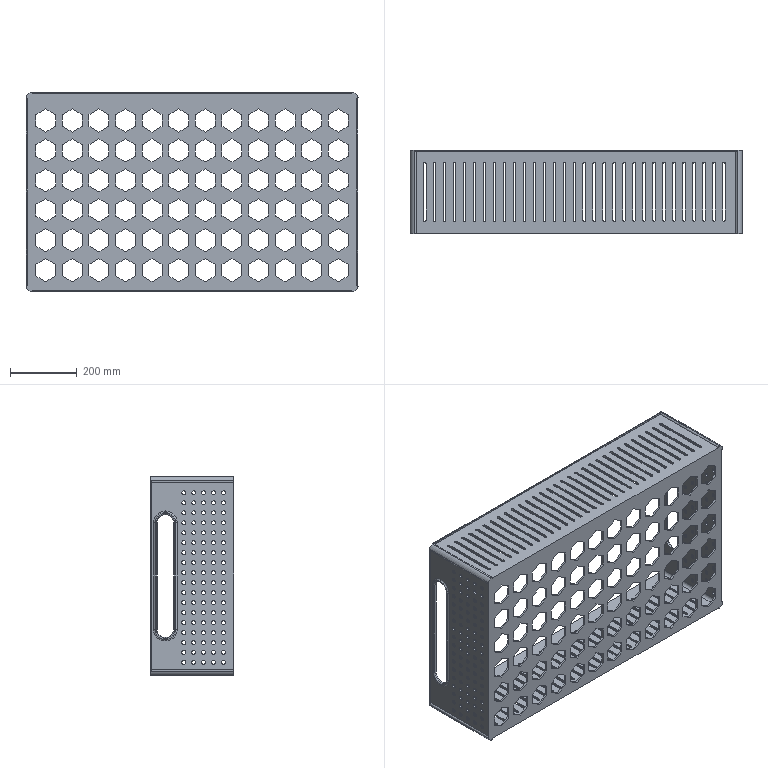Part | SolidWorks | features ICE 12, Fillet 6, Extrusion 1 | 5 solids | 1124 faces | box 998.333 x 250 x 598.333 mm | volume 5087967 mm3 | plane 589 | cylinder 523 | torus 12 | commonest cylinder face diameters 12 x360 8 x124 10 x21 50 x6 6 x4 20 x4